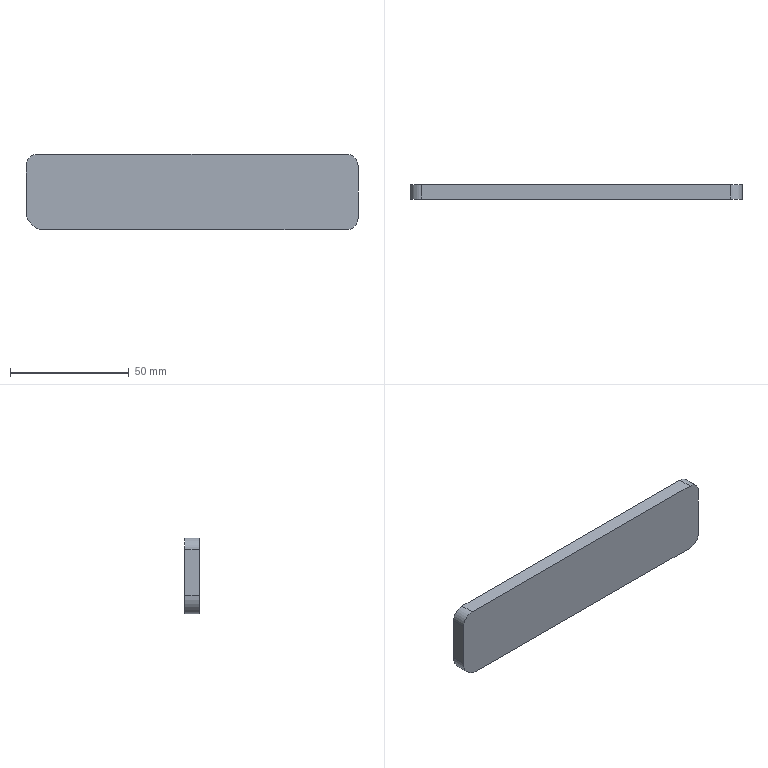Part | STEP file | WEAR-PLATE1_id186_x_t | 1 solid | 10 faces | box 140 x 6 x 32 mm | volume 26706 mm3 | plane 6 | cylinder 4 | commonest cylinder face diameters 10 x3 15.557 x1
STEP:
#1=CARTESIAN_POINT('',(-90.,-66.,69.778));
#2=VERTEX_POINT('',#1);
#3=CARTESIAN_POINT('',(-90.,-66.,89.));
#4=VERTEX_POINT('',#3);
#5=CARTESIAN_POINT('',(-90.,-66.,69.778));
#6=DIRECTION('',(0.,0.,1.));
#7=VECTOR('',#6,1.);
#8=LINE('',#5,#7);
#9=EDGE_CURVE('',#2,#4,#8,.T.);
#10=ORIENTED_EDGE('',*,*,#9,.F.);
#11=CARTESIAN_POINT('',(-82.222,-66.,62.));
#12=VERTEX_POINT('',#11);
#13=CARTESIAN_POINT('',(-82.222,-66.,69.778));
#14=DIRECTION('',(0.,1.,0.));
#15=DIRECTION('',(0.,0.,1.));
#16=AXIS2_PLACEMENT_3D('',#13,#14,#15);
#17=CIRCLE('',#16,7.778);
#18=EDGE_CURVE('',#12,#2,#17,.T.);
#19=ORIENTED_EDGE('',*,*,#18,.F.);
#20=CARTESIAN_POINT('',(45.,-66.,62.));
#21=VERTEX_POINT('',#20);
#22=CARTESIAN_POINT('',(45.,-66.,62.));
#23=DIRECTION('',(-1.,0.,0.));
#24=VECTOR('',#23,1.);
#25=LINE('',#22,#24);
#26=EDGE_CURVE('',#21,#12,#25,.T.);
#27=ORIENTED_EDGE('',*,*,#26,.F.);
#28=CARTESIAN_POINT('',(50.,-66.,67.));
#29=VERTEX_POINT('',#28);
#30=CARTESIAN_POINT('',(45.,-66.,67.));
#31=DIRECTION('',(0.,1.,0.));
#32=DIRECTION('',(0.,0.,1.));
#33=AXIS2_PLACEMENT_3D('',#30,#31,#32);
#34=CIRCLE('',#33,5.);
#35=EDGE_CURVE('',#29,#21,#34,.T.);
#36=ORIENTED_EDGE('',*,*,#35,.F.);
#37=CARTESIAN_POINT('',(50.,-66.,89.));
#38=VERTEX_POINT('',#37);
#39=CARTESIAN_POINT('',(50.,-66.,89.));
#40=DIRECTION('',(0.,0.,-1.));
#41=VECTOR('',#40,1.);
#42=LINE('',#39,#41);
#43=EDGE_CURVE('',#38,#29,#42,.T.);
#44=ORIENTED_EDGE('',*,*,#43,.F.);
#45=CARTESIAN_POINT('',(45.,-66.,94.));
#46=VERTEX_POINT('',#45);
#47=CARTESIAN_POINT('',(45.,-66.,89.));
#48=DIRECTION('',(0.,1.,0.));
#49=DIRECTION('',(0.,0.,1.));
#50=AXIS2_PLACEMENT_3D('',#47,#48,#49);
#51=CIRCLE('',#50,5.);
#52=EDGE_CURVE('',#46,#38,#51,.T.);
#53=ORIENTED_EDGE('',*,*,#52,.F.);
#54=CARTESIAN_POINT('',(-85.,-66.,94.));
#55=VERTEX_POINT('',#54);
#56=CARTESIAN_POINT('',(-85.,-66.,94.));
#57=DIRECTION('',(1.,0.,0.));
#58=VECTOR('',#57,1.);
#59=LINE('',#56,#58);
#60=EDGE_CURVE('',#55,#46,#59,.T.);
#61=ORIENTED_EDGE('',*,*,#60,.F.);
#62=CARTESIAN_POINT('',(-85.,-66.,89.));
#63=DIRECTION('',(0.,1.,0.));
#64=DIRECTION('',(0.,0.,1.));
#65=AXIS2_PLACEMENT_3D('',#62,#63,#64);
#66=CIRCLE('',#65,5.);
#67=EDGE_CURVE('',#4,#55,#66,.T.);
#68=ORIENTED_EDGE('',*,*,#67,.F.);
#69=EDGE_LOOP('',(#10,#19,#27,#36,#44,#53,#61,#68));
#70=FACE_OUTER_BOUND('',#69,.T.);
#71=CARTESIAN_POINT('',(-200.,-66.,-275.));
#72=DIRECTION('',(0.,1.,0.));
#73=DIRECTION('',(0.,0.,1.));
#74=AXIS2_PLACEMENT_3D('',#71,#72,#73);
#75=PLANE('',#74);
#76=ADVANCED_FACE('',(#70),#75,.F.);
#77=CARTESIAN_POINT('',(-85.,-60.,94.));
#78=VERTEX_POINT('',#77);
#79=CARTESIAN_POINT('',(-85.,-66.,94.));
#80=DIRECTION('',(0.,1.,0.));
#81=VECTOR('',#80,1.);
#82=LINE('',#79,#81);
#83=EDGE_CURVE('',#55,#78,#82,.T.);
#84=ORIENTED_EDGE('',*,*,#83,.F.);
#85=ORIENTED_EDGE('',*,*,#60,.T.);
#86=CARTESIAN_POINT('',(45.,-60.,94.));
#87=VERTEX_POINT('',#86);
#88=CARTESIAN_POINT('',(45.,-66.,94.));
#89=DIRECTION('',(0.,-1.,0.));
#90=VECTOR('',#89,1.);
#91=LINE('',#88,#90);
#92=EDGE_CURVE('',#87,#46,#91,.T.);
#93=ORIENTED_EDGE('',*,*,#92,.F.);
#94=CARTESIAN_POINT('',(-80.,-60.,94.));
#95=DIRECTION('',(-1.,0.,0.));
#96=VECTOR('',#95,1.);
#97=LINE('',#94,#96);
#98=EDGE_CURVE('',#87,#78,#97,.T.);
#99=ORIENTED_EDGE('',*,*,#98,.T.);
#100=EDGE_LOOP('',(#84,#85,#93,#99));
#101=FACE_OUTER_BOUND('',#100,.T.);
#102=CARTESIAN_POINT('',(-85.,-66.,94.));
#103=DIRECTION('',(0.,0.,1.));
#104=DIRECTION('',(1.,0.,0.));
#105=AXIS2_PLACEMENT_3D('',#102,#103,#104);
#106=PLANE('',#105);
#107=ADVANCED_FACE('',(#101),#106,.T.);
#108=CARTESIAN_POINT('',(-90.,-60.,89.));
#109=VERTEX_POINT('',#108);
#110=CARTESIAN_POINT('',(-90.,-66.,89.));
#111=DIRECTION('',(0.,1.,0.));
#112=VECTOR('',#111,1.);
#113=LINE('',#110,#112);
#114=EDGE_CURVE('',#4,#109,#113,.T.);
#115=ORIENTED_EDGE('',*,*,#114,.F.);
#116=ORIENTED_EDGE('',*,*,#67,.T.);
#117=ORIENTED_EDGE('',*,*,#83,.T.);
#118=CARTESIAN_POINT('',(-85.,-60.,89.));
#119=DIRECTION('',(0.,-1.,0.));
#120=DIRECTION('',(0.,0.,1.));
#121=AXIS2_PLACEMENT_3D('',#118,#119,#120);
#122=CIRCLE('',#121,5.);
#123=EDGE_CURVE('',#78,#109,#122,.T.);
#124=ORIENTED_EDGE('',*,*,#123,.T.);
#125=EDGE_LOOP('',(#115,#116,#117,#124));
#126=FACE_OUTER_BOUND('',#125,.T.);
#127=CARTESIAN_POINT('',(-85.,-66.,89.));
#128=DIRECTION('',(0.,1.,0.));
#129=DIRECTION('',(0.,0.,1.));
#130=AXIS2_PLACEMENT_3D('',#127,#128,#129);
#131=CYLINDRICAL_SURFACE('',#130,5.);
#132=ADVANCED_FACE('',(#126),#131,.T.);
#133=CARTESIAN_POINT('',(-90.,-60.,69.778));
#134=VERTEX_POINT('',#133);
#135=CARTESIAN_POINT('',(-90.,-66.,69.778));
#136=DIRECTION('',(0.,1.,0.));
#137=VECTOR('',#136,1.);
#138=LINE('',#135,#137);
#139=EDGE_CURVE('',#2,#134,#138,.T.);
#140=ORIENTED_EDGE('',*,*,#139,.F.);
#141=ORIENTED_EDGE('',*,*,#9,.T.);
#142=ORIENTED_EDGE('',*,*,#114,.T.);
#143=CARTESIAN_POINT('',(-90.,-60.,-43.));
#144=DIRECTION('',(0.,0.,-1.));
#145=VECTOR('',#144,1.);
#146=LINE('',#143,#145);
#147=EDGE_CURVE('',#109,#134,#146,.T.);
#148=ORIENTED_EDGE('',*,*,#147,.T.);
#149=EDGE_LOOP('',(#140,#141,#142,#148));
#150=FACE_OUTER_BOUND('',#149,.T.);
#151=CARTESIAN_POINT('',(-90.,-66.,69.778));
#152=DIRECTION('',(-1.,0.,0.));
#153=DIRECTION('',(0.,0.,1.));
#154=AXIS2_PLACEMENT_3D('',#151,#152,#153);
#155=PLANE('',#154);
#156=ADVANCED_FACE('',(#150),#155,.T.);
#157=CARTESIAN_POINT('',(-82.222,-60.,62.));
#158=VERTEX_POINT('',#157);
#159=CARTESIAN_POINT('',(-82.222,-66.,62.));
#160=DIRECTION('',(0.,1.,0.));
#161=VECTOR('',#160,1.);
#162=LINE('',#159,#161);
#163=EDGE_CURVE('',#12,#158,#162,.T.);
#164=ORIENTED_EDGE('',*,*,#163,.F.);
#165=ORIENTED_EDGE('',*,*,#18,.T.);
#166=ORIENTED_EDGE('',*,*,#139,.T.);
#167=CARTESIAN_POINT('',(-82.222,-60.,69.778));
#168=DIRECTION('',(0.,-1.,0.));
#169=DIRECTION('',(0.,0.,1.));
#170=AXIS2_PLACEMENT_3D('',#167,#168,#169);
#171=CIRCLE('',#170,7.778);
#172=EDGE_CURVE('',#134,#158,#171,.T.);
#173=ORIENTED_EDGE('',*,*,#172,.T.);
#174=EDGE_LOOP('',(#164,#165,#166,#173));
#175=FACE_OUTER_BOUND('',#174,.T.);
#176=CARTESIAN_POINT('',(-82.222,-66.,69.778));
#177=DIRECTION('',(0.,1.,0.));
#178=DIRECTION('',(0.,0.,1.));
#179=AXIS2_PLACEMENT_3D('',#176,#177,#178);
#180=CYLINDRICAL_SURFACE('',#179,7.778);
#181=ADVANCED_FACE('',(#175),#180,.T.);
#182=CARTESIAN_POINT('',(45.,-60.,62.));
#183=VERTEX_POINT('',#182);
#184=CARTESIAN_POINT('',(45.,-66.,62.));
#185=DIRECTION('',(0.,1.,0.));
#186=VECTOR('',#185,1.);
#187=LINE('',#184,#186);
#188=EDGE_CURVE('',#21,#183,#187,.T.);
#189=ORIENTED_EDGE('',*,*,#188,.F.);
#190=ORIENTED_EDGE('',*,*,#26,.T.);
#191=ORIENTED_EDGE('',*,*,#163,.T.);
#192=CARTESIAN_POINT('',(-80.,-60.,62.));
#193=DIRECTION('',(1.,0.,0.));
#194=VECTOR('',#193,1.);
#195=LINE('',#192,#194);
#196=EDGE_CURVE('',#158,#183,#195,.T.);
#197=ORIENTED_EDGE('',*,*,#196,.T.);
#198=EDGE_LOOP('',(#189,#190,#191,#197));
#199=FACE_OUTER_BOUND('',#198,.T.);
#200=CARTESIAN_POINT('',(45.,-66.,62.));
#201=DIRECTION('',(0.,0.,-1.));
#202=DIRECTION('',(-1.,0.,0.));
#203=AXIS2_PLACEMENT_3D('',#200,#201,#202);
#204=PLANE('',#203);
#205=ADVANCED_FACE('',(#199),#204,.T.);
#206=CARTESIAN_POINT('',(50.,-60.,67.));
#207=VERTEX_POINT('',#206);
#208=CARTESIAN_POINT('',(50.,-66.,67.));
#209=DIRECTION('',(0.,1.,0.));
#210=VECTOR('',#209,1.);
#211=LINE('',#208,#210);
#212=EDGE_CURVE('',#29,#207,#211,.T.);
#213=ORIENTED_EDGE('',*,*,#212,.F.);
#214=ORIENTED_EDGE('',*,*,#35,.T.);
#215=ORIENTED_EDGE('',*,*,#188,.T.);
#216=CARTESIAN_POINT('',(45.,-60.,67.));
#217=DIRECTION('',(0.,-1.,0.));
#218=DIRECTION('',(0.,0.,1.));
#219=AXIS2_PLACEMENT_3D('',#216,#217,#218);
#220=CIRCLE('',#219,5.);
#221=EDGE_CURVE('',#183,#207,#220,.T.);
#222=ORIENTED_EDGE('',*,*,#221,.T.);
#223=EDGE_LOOP('',(#213,#214,#215,#222));
#224=FACE_OUTER_BOUND('',#223,.T.);
#225=CARTESIAN_POINT('',(45.,-66.,67.));
#226=DIRECTION('',(0.,1.,0.));
#227=DIRECTION('',(0.,0.,1.));
#228=AXIS2_PLACEMENT_3D('',#225,#226,#227);
#229=CYLINDRICAL_SURFACE('',#228,5.);
#230=ADVANCED_FACE('',(#224),#229,.T.);
#231=CARTESIAN_POINT('',(50.,-60.,89.));
#232=VERTEX_POINT('',#231);
#233=CARTESIAN_POINT('',(50.,-66.,89.));
#234=DIRECTION('',(0.,1.,0.));
#235=VECTOR('',#234,1.);
#236=LINE('',#233,#235);
#237=EDGE_CURVE('',#38,#232,#236,.T.);
#238=ORIENTED_EDGE('',*,*,#237,.F.);
#239=ORIENTED_EDGE('',*,*,#43,.T.);
#240=ORIENTED_EDGE('',*,*,#212,.T.);
#241=CARTESIAN_POINT('',(50.,-60.,-43.));
#242=DIRECTION('',(0.,0.,1.));
#243=VECTOR('',#242,1.);
#244=LINE('',#241,#243);
#245=EDGE_CURVE('',#207,#232,#244,.T.);
#246=ORIENTED_EDGE('',*,*,#245,.T.);
#247=EDGE_LOOP('',(#238,#239,#240,#246));
#248=FACE_OUTER_BOUND('',#247,.T.);
#249=CARTESIAN_POINT('',(50.,-66.,89.));
#250=DIRECTION('',(1.,0.,0.));
#251=DIRECTION('',(0.,0.,-1.));
#252=AXIS2_PLACEMENT_3D('',#249,#250,#251);
#253=PLANE('',#252);
#254=ADVANCED_FACE('',(#248),#253,.T.);
#255=ORIENTED_EDGE('',*,*,#92,.T.);
#256=ORIENTED_EDGE('',*,*,#52,.T.);
#257=ORIENTED_EDGE('',*,*,#237,.T.);
#258=CARTESIAN_POINT('',(45.,-60.,89.));
#259=DIRECTION('',(0.,-1.,0.));
#260=DIRECTION('',(0.,0.,1.));
#261=AXIS2_PLACEMENT_3D('',#258,#259,#260);
#262=CIRCLE('',#261,5.);
#263=EDGE_CURVE('',#232,#87,#262,.T.);
#264=ORIENTED_EDGE('',*,*,#263,.T.);
#265=EDGE_LOOP('',(#255,#256,#257,#264));
#266=FACE_OUTER_BOUND('',#265,.T.);
#267=CARTESIAN_POINT('',(45.,-66.,89.));
#268=DIRECTION('',(0.,1.,0.));
#269=DIRECTION('',(0.,0.,1.));
#270=AXIS2_PLACEMENT_3D('',#267,#268,#269);
#271=CYLINDRICAL_SURFACE('',#270,5.);
#272=ADVANCED_FACE('',(#266),#271,.T.);
#273=ORIENTED_EDGE('',*,*,#245,.F.);
#274=ORIENTED_EDGE('',*,*,#221,.F.);
#275=ORIENTED_EDGE('',*,*,#196,.F.);
#276=ORIENTED_EDGE('',*,*,#172,.F.);
#277=ORIENTED_EDGE('',*,*,#147,.F.);
#278=ORIENTED_EDGE('',*,*,#123,.F.);
#279=ORIENTED_EDGE('',*,*,#98,.F.);
#280=ORIENTED_EDGE('',*,*,#263,.F.);
#281=EDGE_LOOP('',(#273,#274,#275,#276,#277,#278,#279,#280));
#282=FACE_OUTER_BOUND('',#281,.T.);
#283=CARTESIAN_POINT('',(-80.,-60.,-43.));
#284=DIRECTION('',(0.,-1.,0.));
#285=DIRECTION('',(0.,0.,-1.));
#286=AXIS2_PLACEMENT_3D('',#283,#284,#285);
#287=PLANE('',#286);
#288=ADVANCED_FACE('',(#282),#287,.F.);
#289=CLOSED_SHELL('',(#76,#107,#132,#156,#181,#205,#230,#254,#272,#288));
#290=MANIFOLD_SOLID_BREP('',#289);
#291=(LENGTH_UNIT()NAMED_UNIT(*)SI_UNIT(.MILLI.,.METRE.));
#292=UNCERTAINTY_MEASURE_WITH_UNIT(LENGTH_MEASURE(0.00002),#291,'','');
#293=(NAMED_UNIT(*)PLANE_ANGLE_UNIT()SI_UNIT($,.RADIAN.));
#294=PLANE_ANGLE_MEASURE_WITH_UNIT(PLANE_ANGLE_MEASURE(0.01745),#293);
#295=DIMENSIONAL_EXPONENTS(0.,0.,0.,0.,0.,0.,0.);
#296=(CONVERSION_BASED_UNIT('DEGREE',#294)NAMED_UNIT(#295)PLANE_ANGLE_UNIT());
#297=(NAMED_UNIT(*)SI_UNIT($,.STERADIAN.)SOLID_ANGLE_UNIT());
#298=(GEOMETRIC_REPRESENTATION_CONTEXT(3)GLOBAL_UNCERTAINTY_ASSIGNED_CONTEXT((#292))GLOBAL_UNIT_ASSIGNED_CONTEXT((#291,#296,#297))REPRESENTATION_CONTEXT('',''));
#299=ADVANCED_BREP_SHAPE_REPRESENTATION('',(#290),#298);